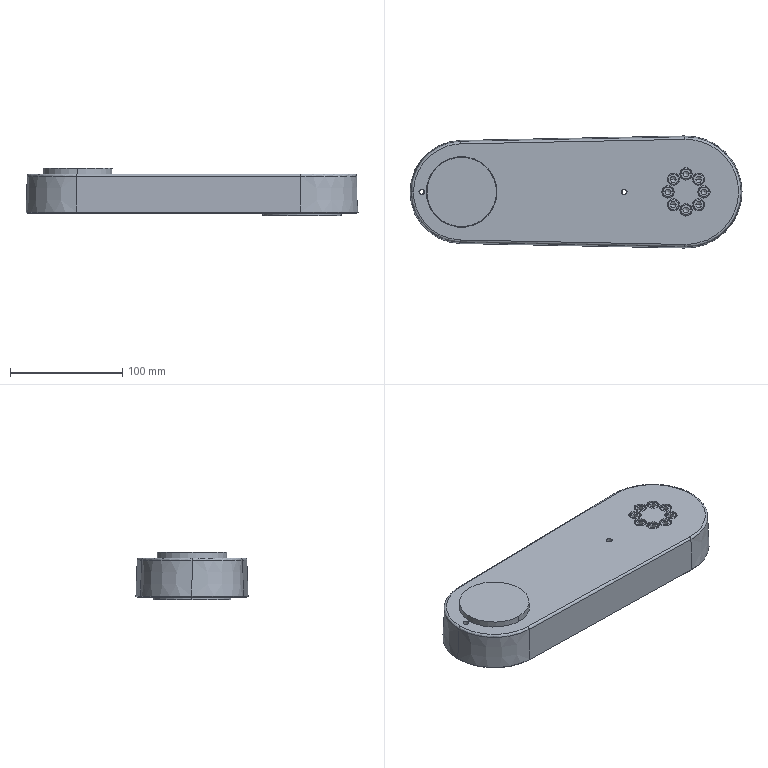Part | STEP file | 11-X arm1111 | 16 solids | 1109 faces | box 295.93 x 99.93 x 42 mm | volume 504380 mm3 | spline 379 | cylinder 335 | plane 272 | cone 62 | torus 61 | commonest cylinder face diameters 10 x116 2 x64 6 x36 4 x16 5 x16 6.6 x16